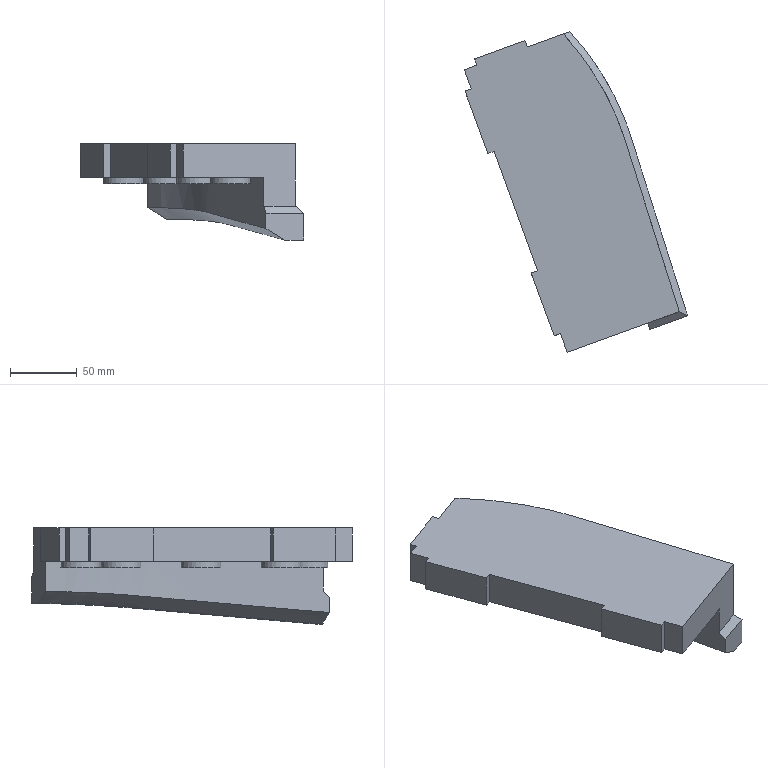Part | NX | features solid 2 | 1 solid | 35 faces | box 167.025 x 240.037 x 71.979 mm | volume 774695 mm3 | plane 24 | spline 6 | cylinder 5 | commonest cylinder face diameters 30 x5